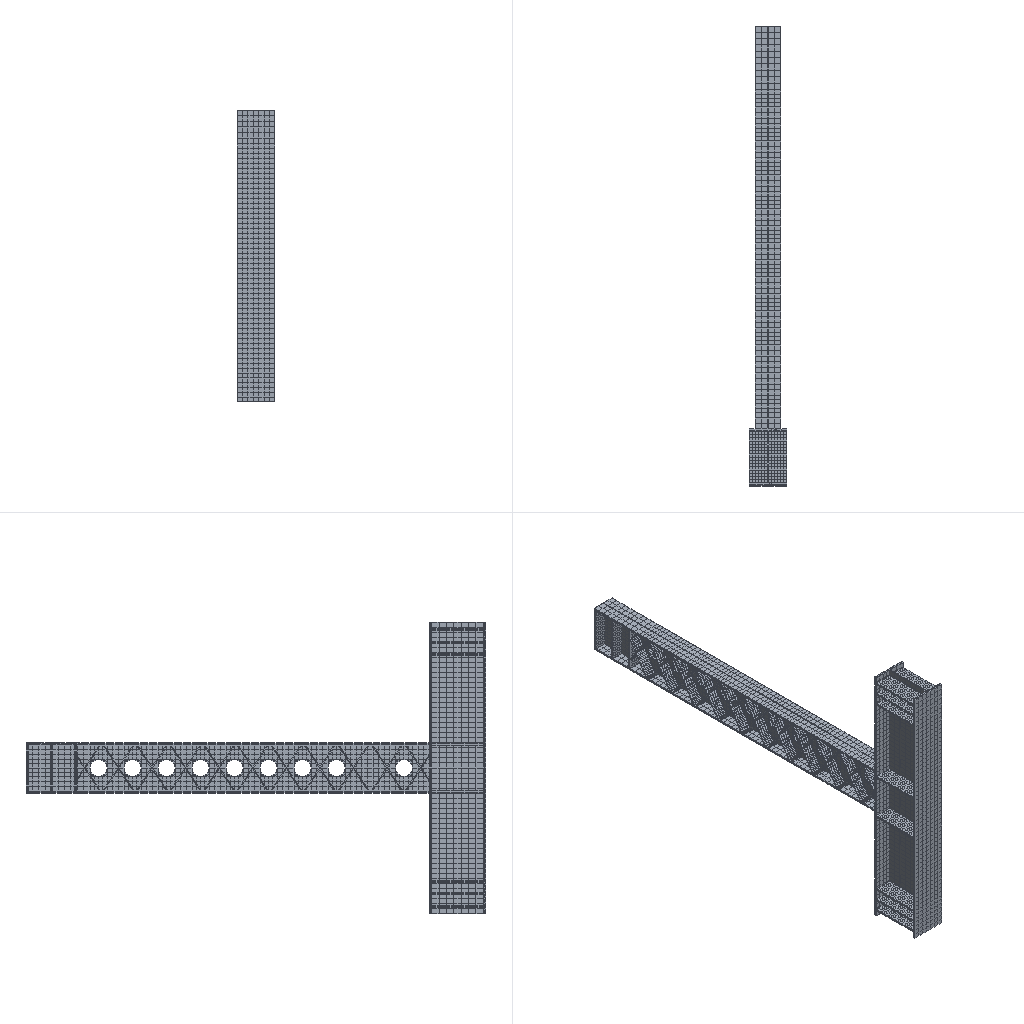Simulation study | abaqus
Set-up summary:
category,name,step,type,value,unit,region
solver,abaqus,,Abaqus/CAE 2024
units,mm-N-s-tonne (MPa),,inferred,E=200000 density=7.85e-09
analysis,Step-1,,buckling,n_modes=5
mesh,nodes,,,29001
mesh,elements,,,16108
element_type,C3D8R,,,16108
material,q235b,,E,200000
material,q235b,,nu,0.2
material,q235b,,density,7.85e-09
material,q235b,,yield,400
material,q235b,,behaviors,plastic
section,q235b,,solid section,,,Set-6
section,q235b,,solid section,,,Set-7
section,q235b,,solid section,,,Set-1
section,q235b,,solid section,,,Set-2
section,q235b,,solid section,,,Set-3
section,q235b,,solid section,,,Set-5
section,q235b,,solid section,,,Set-4
bc,BC-1,initial,fixed,"[dofs=ry,rz,x,y,z n=5]",,Set-4
bc,BC-2,initial,fixed,"[dofs=ry,rz,x,y n=4]",,Set-5
bc,BC-3,initial,fixed,[dofs=x],,Set-9
bc,BC-4,initial,fixed,[dofs=x],,Set-7
bc,BC-1,Step-1,fixed,"[dofs=ry,rz,x,y,z n=5]",,Set-4
bc,,Step-1,fixed,"[dofs=ry,rz,x,y,z n=5]",,Set-4
bc,BC-2,Step-1,fixed,"[dofs=ry,rz,x,y n=4]",,Set-5
bc,,Step-1,fixed,"[dofs=ry,rz,x,y n=4]",,Set-5
bc,BC-3,Step-1,fixed,[dofs=x],,Set-9
bc,,Step-1,fixed,[dofs=x],,Set-9
bc,BC-4,Step-1,fixed,[dofs=x],,Set-7
bc,,Step-1,fixed,[dofs=x],,Set-7
bc,BC-5,Step-1,displacement,-13 [dofs=z],,Set-8
bc,,Step-1,displacement,-13 [dofs=z],,Set-8
contact,Constraint-1,initial,tie,,,_PickedSurf141 / s_Surf-1
contact,Constraint-2,initial,tie,,,_PickedSurf142 / s_Surf-3
contact,Constraint-3,initial,tie,,,_PickedSurf143 / s_Surf-5
contact,Constraint-4,initial,tie,,,s_Surf-7 / m_Surf-7
contact,Constraint-5,initial,tie,,,s_Surf-9 / m_Surf-9
contact,Constraint-10,initial,tie,,,Surf-15 / s_Surf-5
contact,Constraint-11,initial,tie,,,s_Surf-20 / Surf-16
contact,Constraint-12,initial,tie,,,Surf-18 / s_Surf-24
contact,Constraint-13,initial,tie,,,s_Surf-5 / Surf-19
contact,Constraint-14,initial,tie,,,s_Surf-25 / Surf-20
contact,Constraint-15,initial,tie,,,Surf-23 / s_Surf-17
constraint,coupling,,,3
Abaqus input file, long lists of numbers shortened:
*Heading
** Job name: deck Model name: buqiangban-13-motai
** Generated by: Abaqus/CAE 2024
*Preprint, echo=NO, model=NO, history=NO, contact=NO
**
** PARTS
**
*Part, name=Part-1
*Node
      1,         154.,         511.,        1158.
      2,         250.,         511.,        1158.
** (463 more lines like these left out)
*Element, type=C3D8R
 1,  54, 201, 385, 193,   1,  25, 169,  38
 2, 201, 202, 386, 385,  25,  26, 170, 169
** (238 more lines like these left out)
*Nset, nset=Set-6, generate
   1,  465,    1
*Elset, elset=Set-6, generate
   1,  240,    1
** Section: q235b
*Solid Section, elset=Set-6, material=q235b
,
*End Part
**
*Part, name=Part-22
*Node
      1,         154.,   779.425,        1158.
      2,         250.,   779.425,        1158.
** (553 more lines like these left out)
*Element, type=C3D8R
 1,  66, 249, 457, 235,   1,  25, 193,  44
 2, 249, 250, 458, 457,  25,  26, 194, 193
** (286 more lines like these left out)
*Nset, nset=Set-7, generate
   1,  555,    1
*Elset, elset=Set-7, generate
   1,  288,    1
** Section: q235b
*Solid Section, elset=Set-7, material=q235b
,
*End Part
**
*Part, name=h400
*Node
      1,           0.,          16.,        507.5
      2,          96.,          16.,        507.5
** (5923 more lines like these left out)
*Element, type=C3D8R
 1,  631, 2752, 5141, 2734,    1,  590, 2716,  609
 2, 2752,  633, 2743, 5141,  590,    2,  591, 2716
** (3618 more lines like these left out)
*Nset, nset=Set-1, generate
    1,  5925,     1
*Elset, elset=Set-1, generate
    1,  3620,     1
** Section: q235b
*Solid Section, elset=Set-1, material=q235b
,
*End Part
**
*Part, name=h450
*Node
      1,         155.,         430.,        2316.
      2,         155.,          20.,        2316.
** (4069 more lines like these left out)
*Element, type=C3D8R
  1,  282, 1595, 2989, 1481,    1,   29,  797,  154
  2, 1595, 1596, 2990, 2989,   29,   30,  798,  797
** (2550 more lines like these left out)
*Nset, nset=Set-2, generate
    1,  4071,     1
*Elset, elset=Set-2, generate
    1,  2552,     1
** Section: q235b
*Solid Section, elset=Set-2, material=q235b
,
*End Part
**
*Part, name=jiajinlei20
*Node
      1,          96.,         368.,          20.
      2,          96.,   343.467,          20.
** (238 more lines like these left out)
*Element, type=C3D8R
  1,  49,  50,  66,  65,   1,   2,  18,  17
  2,  50,  51,  67,  66,   2,   3,  19,  18
** (118 more lines like these left out)
*Nset, nset=Set-3, generate
   1,  240,    1
*Elset, elset=Set-3, generate
   1,  120,    1
** Section: q235b
*Solid Section, elset=Set-3, material=q235b
,
*End Part
**
*Part, name=jiajinlei20di
*Node
      1,        112.5,         225.,          20.
      2,        112.5,      199.375,          20.
** (355 more lines like these left out)
*Element, type=C3D8R
  1,  52,  53,  70,  69,   1,   2,  19,  18
  2,  53,  54,  71,  70,   2,   3,  20,  19
** (190 more lines like these left out)
*Nset, nset=Set-5, generate
   1,  357,    1
*Elset, elset=Set-5, generate
   1,  192,    1
** Section: q235b
*Solid Section, elset=Set-5, material=q235b
,
*End Part
**
*Part, name=jiajinlie16
*Node
      1,        187.5,         375.,          16.
      2,        187.5,      349.375,          16.
** (355 more lines like these left out)
*Element, type=C3D8R
  1,  52,  53,  70,  69,   1,   2,  19,  18
  2,  53,  54,  71,  70,   2,   3,  20,  19
** (190 more lines like these left out)
*Nset, nset=Set-4, generate
   1,  357,    1
*Elset, elset=Set-4, generate
   1,  192,    1
** Section: q235b
*Solid Section, elset=Set-4, material=q235b
,
*End Part
**
**
** ASSEMBLY
**
*Assembly, name=Assembly
**
*Instance, name=h450, part=h450
*End Instance
**
*Instance, name=jiajinlie16-1, part=jiajinlie16
       112.5,          55.,        2250.
*End Instance
**
*Instance, name=jiajinlie16-1-lin-1-2, part=jiajinlie16
       112.5,          55.,        2150.
*End Instance
**
*Instance, name=jiajinlie16-1-lin-1-3, part=jiajinlie16
       112.5,          55.,        2050.
*End Instance
**
*Instance, name=jiajinlie16-1-lin-1-6, part=jiajinlie16
       112.5,          55.,          50.
*End Instance
**
*Instance, name=jiajinlie16-1-lin-1-7, part=jiajinlie16
       112.5,          55.,         150.
*End Instance
**
*Instance, name=jiajinlie16-1-lin-1-8, part=jiajinlie16
       112.5,          55.,         250.
*End Instance
**
*Instance, name=jiajinlie16-1-lin-1-2-1, part=jiajinlie16
       -42.5,          55.,        2250.
*End Instance
**
*Instance, name=jiajinlie16-1-lin-1-2-lin-1-2, part=jiajinlie16
       -42.5,          55.,        2150.
*End Instance
**
*Instance, name=jiajinlie16-1-lin-1-8-lin-1-2, part=jiajinlie16
       -42.5,          55.,         250.
*End Instance
**
*Instance, name=jiajinlie16-1-lin-1-6-lin-1-2, part=jiajinlie16
       -42.5,          55.,          50.
*End Instance
**
*Instance, name=jiajinlie16-1-lin-1-3-lin-1-2, part=jiajinlie16
       -42.5,          55.,        2050.
*End Instance
**
*Instance, name=jiajinlie16-1-lin-1-7-lin-1-2, part=jiajinlie16
       -42.5,          55.,         150.
*End Instance
**
*Instance, name=h400, part=h400
         50.,        3650.,         958.
         50.,        3650.,         958., 51.,        3650.,         958., 90.
*End Instance
**
*Instance, name=jiajinlei20-1, part=jiajinlei20
        154.,        3650.,         974.
        154.,        3650.,         974., 155.,        3650.,         974., 90.
*End Instance
**
*Instance, name=jiajinlei20-1-lin-1-2, part=jiajinlei20
        154.,        3460.,         974.
        154.,        3460.,         974., 155.,        3460.,         974., 90.
*End Instance
**
*Instance, name=jiajinlei20-1-lin-1-3, part=jiajinlei20
        154.,        3270.,         974.
        154.,        3270.,         974., 155.,        3270.,         974., 90.
*End Instance
**
*Instance, name=jiajinlei20-1-lin-1-2-1, part=jiajinlei20
         50.,        3650.,         974.
         50.,        3650.,         974., 51.,        3650.,         974., 90.
*End Instance
**
*Instance, name=jiajinlei20-1-lin-1-2-lin-1-2, part=jiajinlei20
         50.,        3460.,         974.
         50.,        3460.,         974., 51.,        3460.,         974., 90.
*End Instance
**
*Instance, name=jiajinlei20-1-lin-1-3-lin-1-2, part=jiajinlei20
         50.,        3270.,         974.
         50.,        3270.,         974., 51.,        3270.,         974., 90.
*End Instance
**
*Instance, name=Part-1-1, part=Part-1
*End Instance
**
*Instance, name=Part-22-1, part=Part-22
*End Instance
**
*Instance, name=Part-22-1-lin-2-1, part=Part-22
          0.,     266.575,           0.
*End Instance
**
*Instance, name=Part-22-1-lin-2-1-lin-2-1, part=Part-22
          0.,     533.15,           0.
*End Instance
**
*Instance, name=Part-22-1-lin-2-1-lin-3-1, part=Part-22
          0.,     799.724,           0.
*End Instance
**
*Instance, name=Part-22-1-lin-2-1-lin-4-1, part=Part-22
          0.,    1066.299,           0.
*End Instance
**
*Instance, name=Part-22-1-lin-2-1-lin-5-1, part=Part-22
          0.,     1332.874,           0.
*End Instance
**
*Instance, name=Part-22-1-lin-2-1-lin-6-1, part=Part-22
          0.,    1599.449,           0.
*End Instance
**
*Instance, name=Part-22-1-lin-2-1-lin-7-1, part=Part-22
          0.,    1866.024,           0.
*End Instance
**
*Instance, name=Part-22-1-lin-2-1-lin-8-1, part=Part-22
          0.,    2132.598,           0.
*End Instance
**
*Instance, name=Part-1-2, part=Part-1
        404.,        3700.,           0.
        404.,        3700.,           0.,         404.,        3700.,           1.,         180.
*End Instance
**
*Instance, name=Part-1-2-lin-1-2, part=Part-1
        300.,        3700.,           0.
        300.,        3700.,           0.,         300.,        3700.,           1.,         180.
*End Instance
**
*Instance, name=Part-22-1-lin-2-1-lin-8-1-lin-1-2, part=Part-22
       -104.,    2132.598,           0.
*End Instance
**
*Instance, name=Part-22-1-lin-2-1-lin-7-1-lin-1-2, part=Part-22
       -104.,    1866.024,           0.
*End Instance
**
*Instance, name=Part-22-1-lin-2-1-lin-6-1-lin-1-2, part=Part-22
       -104.,    1599.449,           0.
*End Instance
**
*Instance, name=Part-22-1-lin-2-1-lin-5-1-lin-1-2, part=Part-22
       -104.,     1332.874,           0.
*End Instance
**
*Instance, name=Part-22-1-lin-2-1-lin-4-1-lin-1-2, part=Part-22
       -104.,    1066.299,           0.
*End Instance
**
*Instance, name=Part-22-1-lin-2-1-lin-2-1-lin-1-2, part=Part-22
       -104.,     533.15,           0.
*End Instance
**
*Instance, name=Part-22-1-lin-1-2, part=Part-22
       -104.,           0.,           0.
*End Instance
**
*Instance, name=Part-22-1-lin-2-1-lin-1-2, part=Part-22
       -104.,     266.575,           0.
*End Instance
**
*Instance, name=Part-22-1-lin-2-1-lin-3-1-lin-1-2, part=Part-22
       -104.,     799.724,           0.
*End Instance
**
*Instance, name=Part-1-1-lin-1-2, part=Part-1
       -104.,           0.,           0.
*End Instance
**
*Instance, name=jiajinlei20di-1, part=jiajinlei20di
       187.5,         205.,        1340.
*End Instance
**
*Instance, name=jiajinlei20di-2, part=jiajinlei20di
       187.5,         205.,         956.
*End Instance
**
*Instance, name=jiajinlei20di-1-lin-1-2, part=jiajinlei20di
        32.5,         205.,        1340.
*End Instance
**
*Instance, name=jiajinlei20di-2-lin-1-2, part=jiajinlei20di
        32.5,         205.,         956.
*End Instance
**
*Node
      1,         150.,           0.,        2183.
*Node
      2,         150.,           0.,         133.
*Node
      3,         150.,        3450.,        1358.
*Nset, nset=Set-4
 1,
*Nset, nset=Set-5
 2,
*Nset, nset=Set-6, instance=jiajinlie16-1, generate
  1,  51,   1
*Nset, nset=Set-6, instance=jiajinlie16-1-lin-1-2, generate
  1,  51,   1
*Nset, nset=Set-6, instance=jiajinlie16-1-lin-1-3, generate
  1,  51,   1
*Nset, nset=Set-6, instance=jiajinlie16-1-lin-1-7, generate
  1,  51,   1
*Nset, nset=Set-6, instance=jiajinlie16-1-lin-1-2-1, generate
 307,  357,    1
*Nset, nset=Set-6, instance=jiajinlie16-1-lin-1-6-lin-1-2, generate
 307,  357,    1
*Nset, nset=Set-6, instance=jiajinlie16-1-lin-1-6, generate
  1,  51,   1
*Nset, nset=Set-6, instance=jiajinlie16-1-lin-1-8, generate
  1,  51,   1
*Nset, nset=Set-6, instance=jiajinlie16-1-lin-1-7-lin-1-2, generate
 307,  357,    1
*Nset, nset=Set-6, instance=jiajinlie16-1-lin-1-8-lin-1-2, generate
 307,  357,    1
*Nset, nset=Set-6, instance=jiajinlie16-1-lin-1-2-lin-1-2, generate
 307,  357,    1
*Nset, nset=Set-6, instance=jiajinlie16-1-lin-1-3-lin-1-2, generate
 307,  357,    1
*Elset, elset=Set-6, instance=jiajinlie16-1, generate
  1,  32,   1
*Elset, elset=Set-6, instance=jiajinlie16-1-lin-1-2, generate
  1,  32,   1
*Elset, elset=Set-6, instance=jiajinlie16-1-lin-1-3, generate
  1,  32,   1
*Elset, elset=Set-6, instance=jiajinlie16-1-lin-1-7, generate
  1,  32,   1
*Elset, elset=Set-6, instance=jiajinlie16-1-lin-1-2-1, generate
 161,  192,    1
*Elset, elset=Set-6, instance=jiajinlie16-1-lin-1-6-lin-1-2, generate
 161,  192,    1
*Elset, elset=Set-6, instance=jiajinlie16-1-lin-1-6, generate
  1,  32,   1
*Elset, elset=Set-6, instance=jiajinlie16-1-lin-1-8, generate
  1,  32,   1
*Elset, elset=Set-6, instance=jiajinlie16-1-lin-1-7-lin-1-2, generate
 161,  192,    1
*Elset, elset=Set-6, instance=jiajinlie16-1-lin-1-8-lin-1-2, generate
 161,  192,    1
*Elset, elset=Set-6, instance=jiajinlie16-1-lin-1-2-lin-1-2, generate
 161,  192,    1
*Elset, elset=Set-6, instance=jiajinlie16-1-lin-1-3-lin-1-2, generate
 161,  192,    1
*Nset, nset=Set-7, instance=jiajinlei20-1, generate
  1,  48,   1
*Nset, nset=Set-7, instance=jiajinlei20-1-lin-1-2, generate
  1,  48,   1
*Nset, nset=Set-7, instance=jiajinlei20-1-lin-1-2-1, generate
 193,  240,    1
*Nset, nset=Set-7, instance=jiajinlei20-1-lin-1-3-lin-1-2, generate
 193,  240,    1
*Nset, nset=Set-7, instance=jiajinlei20-1-lin-1-3, generate
  1,  48,   1
*Nset, nset=Set-7, instance=jiajinlei20-1-lin-1-2-lin-1-2, generate
 193,  240,    1
*Elset, elset=Set-7, instance=jiajinlei20-1, generate
  1,  30,   1
*Elset, elset=Set-7, instance=jiajinlei20-1-lin-1-2, generate
  1,  30,   1
*Elset, elset=Set-7, instance=jiajinlei20-1-lin-1-2-1, generate
  91,  120,    1
*Elset, elset=Set-7, instance=jiajinlei20-1-lin-1-3-lin-1-2, generate
  91,  120,    1
*Elset, elset=Set-7, instance=jiajinlei20-1-lin-1-3, generate
  1,  30,   1
*Elset, elset=Set-7, instance=jiajinlei20-1-lin-1-2-lin-1-2, generate
  91,  120,    1
*Nset, nset=Set-8
 3,
*Nset, nset=Set-9, instance=jiajinlie16-1, generate
  1,  51,   1
*Nset, nset=Set-9, instance=jiajinlie16-1-lin-1-2, generate
  1,  51,   1
*Nset, nset=Set-9, instance=jiajinlie16-1-lin-1-3, generate
  1,  51,   1
*Nset, nset=Set-9, instance=jiajinlie16-1-lin-1-7, generate
  1,  51,   1
*Nset, nset=Set-9, instance=jiajinlie16-1-lin-1-2-1, generate
 307,  357,    1
*Nset, nset=Set-9, instance=jiajinlie16-1-lin-1-6-lin-1-2, generate
 307,  357,    1
*Nset, nset=Set-9, instance=jiajinlie16-1-lin-1-6, generate
  1,  51,   1
*Nset, nset=Set-9, instance=jiajinlie16-1-lin-1-8, generate
  1,  51,   1
*Nset, nset=Set-9, instance=jiajinlie16-1-lin-1-7-lin-1-2, generate
 307,  357,    1
*Nset, nset=Set-9, instance=jiajinlie16-1-lin-1-8-lin-1-2, generate
 307,  357,    1
*Nset, nset=Set-9, instance=jiajinlie16-1-lin-1-2-lin-1-2, generate
 307,  357,    1
*Nset, nset=Set-9, instance=jiajinlie16-1-lin-1-3-lin-1-2, generate
 307,  357,    1
*Nset, nset=Set-9, instance=jiajinlei20di-1, generate
  1,  51,   1
*Nset, nset=Set-9, instance=jiajinlei20di-1-lin-1-2, generate
 307,  357,    1
*Nset, nset=Set-9, instance=jiajinlei20di-2, generate
  1,  51,   1
*Nset, nset=Set-9, instance=jiajinlei20di-2-lin-1-2, generate
 307,  357,    1
*Elset, elset=Set-9, instance=jiajinlie16-1, generate
  1,  32,   1
*Elset, elset=Set-9, instance=jiajinlie16-1-lin-1-2, generate
  1,  32,   1
*Elset, elset=Set-9, instance=jiajinlie16-1-lin-1-3, generate
  1,  32,   1
*Elset, elset=Set-9, instance=jiajinlie16-1-lin-1-7, generate
  1,  32,   1
*Elset, elset=Set-9, instance=jiajinlie16-1-lin-1-2-1, generate
 161,  192,    1
*Elset, elset=Set-9, instance=jiajinlie16-1-lin-1-6-lin-1-2, generate
 161,  192,    1
*Elset, elset=Set-9, instance=jiajinlie16-1-lin-1-6, generate
  1,  32,   1
*Elset, elset=Set-9, instance=jiajinlie16-1-lin-1-8, generate
  1,  32,   1
*Elset, elset=Set-9, instance=jiajinlie16-1-lin-1-7-lin-1-2, generate
 161,  192,    1
*Elset, elset=Set-9, instance=jiajinlie16-1-lin-1-8-lin-1-2, generate
 161,  192,    1
*Elset, elset=Set-9, instance=jiajinlie16-1-lin-1-2-lin-1-2, generate
 161,  192,    1
*Elset, elset=Set-9, instance=jiajinlie16-1-lin-1-3-lin-1-2, generate
 161,  192,    1
*Elset, elset=Set-9, instance=jiajinlei20di-1, generate
  1,  32,   1
*Elset, elset=Set-9, instance=jiajinlei20di-1-lin-1-2, generate
 161,  192,    1
*Elset, elset=Set-9, instance=jiajinlei20di-2, generate
  1,  32,   1
*Elset, elset=Set-9, instance=jiajinlei20di-2-lin-1-2, generate
 161,  192,    1
*Nset, nset=m_Set-1
 3,
*Nset, nset=m_Set-2
 1,
*Nset, nset=m_Set-3
 2,
*Elset, elset=_Surf-15_S5, internal, instance=Part-1-1
  17,  18,  19,  20,  37,  38,  39,  40, 173, 174, 175, 176, 237, 238, 239, 240
*Surface, type=ELEMENT, name=Surf-15
_Surf-15_S5, S5
*Elset, elset=_Surf-16_S5, internal, instance=Part-1-2
  17,  18,  19,  20,  37,  38,  39,  40, 173, 174, 175, 176, 237, 238, 239, 240
*Surface, type=ELEMENT, name=Surf-16
_Surf-16_S5, S5
*Elset, elset=_Surf-18_S4, internal, instance=Part-1-2-lin-1-2, generate
  44,  240,    4
*Elset, elset=_Surf-18_S4, internal, instance=Part-22-1-lin-2-1-lin-8-1-lin-1-2, generate
   4,  216,    4
*Elset, elset=_Surf-18_S4, internal, instance=Part-22-1-lin-2-1-lin-6-1-lin-1-2, generate
   4,  216,    4
*Elset, elset=_Surf-18_S4, internal, instance=Part-22-1-lin-2-1-lin-4-1-lin-1-2, generate
   4,  216,    4
*Elset, elset=_Surf-18_S4, internal, instance=Part-22-1-lin-2-1-lin-3-1-lin-1-2, generate
   4,  216,    4
*Elset, elset=_Surf-18_S4, internal, instance=Part-22-1-lin-1-2, generate
   4,  216,    4
*Elset, elset=_Surf-18_S4, internal, instance=Part-22-1-lin-2-1-lin-7-1-lin-1-2, generate
   4,  216,    4
*Elset, elset=_Surf-18_S4, internal, instance=Part-22-1-lin-2-1-lin-2-1-lin-1-2, generate
   4,  216,    4
*Elset, elset=_Surf-18_S4, internal, instance=Part-1-1-lin-1-2, generate
  4,  40,   4
*Elset, elset=_Surf-18_S4, internal, instance=Part-22-1-lin-2-1-lin-5-1-lin-1-2, generate
   4,  216,    4
*Elset, elset=_Surf-18_S4, internal, instance=Part-22-1-lin-2-1-lin-1-2, generate
   4,  216,    4
*Elset, elset=_Surf-18_S3, internal, instance=Part-1-2-lin-1-2
 113, 114, 115, 116, 177, 178, 179, 180
*Elset, elset=_Surf-18_S3, internal, instance=Part-22-1-lin-2-1-lin-8-1-lin-1-2
  65,  66,  67,  68, 141, 142, 143, 144
*Elset, elset=_Surf-18_S3, internal, instance=Part-22-1-lin-2-1-lin-6-1-lin-1-2
  65,  66,  67,  68, 141, 142, 143, 144
*Elset, elset=_Surf-18_S3, internal, instance=Part-22-1-lin-2-1-lin-4-1-lin-1-2
  65,  66,  67,  68, 141, 142, 143, 144
*Elset, elset=_Surf-18_S3, internal, instance=Part-22-1-lin-2-1-lin-3-1-lin-1-2
  65,  66,  67,  68, 141, 142, 143, 144
*Elset, elset=_Surf-18_S3, internal, instance=Part-22-1-lin-1-2
  65,  66,  67,  68, 141, 142, 143, 144
*Elset, elset=_Surf-18_S3, internal, instance=Part-22-1-lin-2-1-lin-7-1-lin-1-2
  65,  66,  67,  68, 141, 142, 143, 144
*Elset, elset=_Surf-18_S3, internal, instance=Part-22-1-lin-2-1-lin-2-1-lin-1-2
  65,  66,  67,  68, 141, 142, 143, 144
*Elset, elset=_Surf-18_S3, internal, instance=Part-1-1-lin-1-2
 113, 114, 115, 116, 177, 178, 179, 180
*Elset, elset=_Surf-18_S3, internal, instance=Part-22-1-lin-2-1-lin-5-1-lin-1-2
  65,  66,  67,  68, 141, 142, 143, 144
*Elset, elset=_Surf-18_S3, internal, instance=Part-22-1-lin-2-1-lin-1-2
  65,  66,  67,  68, 141, 142, 143, 144
*Elset, elset=_Surf-18_S5, internal, instance=Part-1-2-lin-1-2
  73,  74,  75,  76, 109, 110, 111, 112
*Elset, elset=_Surf-18_S5, internal, instance=Part-22-1-lin-2-1-lin-8-1-lin-1-2
  29,  30,  31,  32,  61,  62,  63,  64, 137, 138, 139, 140, 213, 214, 215, 216
 249, 250, 251, 252, 285, 286, 287, 288
*Elset, elset=_Surf-18_S5, internal, instance=Part-22-1-lin-2-1-lin-6-1-lin-1-2
  29,  30,  31,  32,  61,  62,  63,  64, 137, 138, 139, 140, 213, 214, 215, 216
 249, 250, 251, 252, 285, 286, 287, 288
*Elset, elset=_Surf-18_S5, internal, instance=Part-22-1-lin-2-1-lin-4-1-lin-1-2
  29,  30,  31,  32,  61,  62,  63,  64, 137, 138, 139, 140, 213, 214, 215, 216
 249, 250, 251, 252, 285, 286, 287, 288
*Elset, elset=_Surf-18_S5, internal, instance=Part-22-1-lin-2-1-lin-3-1-lin-1-2
  29,  30,  31,  32,  61,  62,  63,  64, 137, 138, 139, 140, 213, 214, 215, 216
 249, 250, 251, 252, 285, 286, 287, 288
*Elset, elset=_Surf-18_S5, internal, instance=Part-22-1-lin-1-2
  29,  30,  31,  32,  61,  62,  63,  64, 137, 138, 139, 140, 213, 214, 215, 216
 249, 250, 251, 252, 285, 286, 287, 288
*Elset, elset=_Surf-18_S5, internal, instance=Part-22-1-lin-2-1-lin-7-1-lin-1-2
  29,  30,  31,  32,  61,  62,  63,  64, 137, 138, 139, 140, 213, 214, 215, 216
 249, 250, 251, 252, 285, 286, 287, 288
*Elset, elset=_Surf-18_S5, internal, instance=Part-22-1-lin-2-1-lin-2-1-lin-1-2
  29,  30,  31,  32,  61,  62,  63,  64, 137, 138, 139, 140, 213, 214, 215, 216
 249, 250, 251, 252, 285, 286, 287, 288
*Elset, elset=_Surf-18_S5, internal, instance=Part-1-1-lin-1-2
  73,  74,  75,  76, 109, 110, 111, 112
*Elset, elset=_Surf-18_S5, internal, instance=Part-22-1-lin-2-1-lin-5-1-lin-1-2
  29,  30,  31,  32,  61,  62,  63,  64, 137, 138, 139, 140, 213, 214, 215, 216
 249, 250, 251, 252, 285, 286, 287, 288
*Elset, elset=_Surf-18_S5, internal, instance=Part-22-1-lin-2-1-lin-1-2
  29,  30,  31,  32,  61,  62,  63,  64, 137, 138, 139, 140, 213, 214, 215, 216
 249, 250, 251, 252, 285, 286, 287, 288
*Elset, elset=_Surf-18_S6, internal, instance=Part-1-2-lin-1-2, generate
  1,  37,   4
*Elset, elset=_Surf-18_S6, internal, instance=Part-22-1-lin-2-1-lin-8-1-lin-1-2, generate
 217,  285,    4
*Elset, elset=_Surf-18_S6, internal, instance=Part-22-1-lin-2-1-lin-6-1-lin-1-2, generate
 217,  285,    4
*Elset, elset=_Surf-18_S6, internal, instance=Part-22-1-lin-2-1-lin-4-1-lin-1-2, generate
 217,  285,    4
*Elset, elset=_Surf-18_S6, internal, instance=Part-22-1-lin-2-1-lin-3-1-lin-1-2, generate
 217,  285,    4
*Elset, elset=_Surf-18_S6, internal, instance=Part-22-1-lin-1-2, generate
 217,  285,    4
*Elset, elset=_Surf-18_S6, internal, instance=Part-22-1-lin-2-1-lin-7-1-lin-1-2, generate
 217,  285,    4
*Elset, elset=_Surf-18_S6, internal, instance=Part-22-1-lin-2-1-lin-2-1-lin-1-2, generate
 217,  285,    4
*Elset, elset=_Surf-18_S6, internal, instance=Part-1-1-lin-1-2, generate
  41,  237,    4
*Elset, elset=_Surf-18_S6, internal, instance=Part-22-1-lin-2-1-lin-5-1-lin-1-2, generate
 217,  285,    4
*Elset, elset=_Surf-18_S6, internal, instance=Part-22-1-lin-2-1-lin-1-2, generate
 217,  285,    4
*Surface, type=ELEMENT, name=Surf-18
_Surf-18_S4, S4
_Surf-18_S3, S3
_Surf-18_S6, S6
_Surf-18_S5, S5
*Elset, elset=_Surf-19_S5, internal, instance=Part-1-1-lin-1-2
  17,  18,  19,  20,  37,  38,  39,  40, 173, 174, 175, 176, 237, 238, 239, 240
*Surface, type=ELEMENT, name=Surf-19
_Surf-19_S5, S5
*Elset, elset=_Surf-20_S5, internal, instance=Part-1-2-lin-1-2
  17,  18,  19,  20,  37,  38,  39,  40, 173, 174, 175, 176, 237, 238, 239, 240
*Surface, type=ELEMENT, name=Surf-20
_Surf-20_S5, S5
*Elset, elset=_Surf-23_S4, internal, instance=Part-1-1, generate
  44,  240,    4
*Elset, elset=_Surf-23_S4, internal, instance=Part-22-1, generate
 220,  288,    4
*Elset, elset=_Surf-23_S4, internal, instance=Part-22-1-lin-2-1, generate
 220,  288,    4
*Elset, elset=_Surf-23_S4, internal, instance=Part-22-1-lin-2-1-lin-3-1, generate
 220,  288,    4
*Elset, elset=_Surf-23_S4, internal, instance=Part-22-1-lin-2-1-lin-7-1, generate
 220,  288,    4
*Elset, elset=_Surf-23_S4, internal, instance=Part-22-1-lin-2-1-lin-5-1, generate
 220,  288,    4
*Elset, elset=_Surf-23_S4, internal, instance=Part-1-2, generate
  4,  40,   4
*Elset, elset=_Surf-23_S4, internal, instance=Part-22-1-lin-2-1-lin-2-1, generate
 220,  288,    4
*Elset, elset=_Surf-23_S4, internal, instance=Part-22-1-lin-2-1-lin-4-1, generate
 220,  288,    4
*Elset, elset=_Surf-23_S4, internal, instance=Part-22-1-lin-2-1-lin-8-1, generate
 220,  288,    4
*Elset, elset=_Surf-23_S4, internal, instance=Part-22-1-lin-2-1-lin-6-1, generate
 220,  288,    4
*Elset, elset=_Surf-23_S3, internal, instance=Part-1-1
 113, 114, 115, 116, 177, 178, 179, 180
*Elset, elset=_Surf-23_S3, internal, instance=Part-22-1
  65,  66,  67,  68, 141, 142, 143, 144
*Elset, elset=_Surf-23_S3, internal, instance=Part-22-1-lin-2-1
  65,  66,  67,  68, 141, 142, 143, 144
*Elset, elset=_Surf-23_S3, internal, instance=Part-22-1-lin-2-1-lin-3-1
  65,  66,  67,  68, 141, 142, 143, 144
*Elset, elset=_Surf-23_S3, internal, instance=Part-22-1-lin-2-1-lin-7-1
  65,  66,  67,  68, 141, 142, 143, 144
*Elset, elset=_Surf-23_S3, internal, instance=Part-22-1-lin-2-1-lin-5-1
  65,  66,  67,  68, 141, 142, 143, 144
*Elset, elset=_Surf-23_S3, internal, instance=Part-1-2
 113, 114, 115, 116, 177, 178, 179, 180
*Elset, elset=_Surf-23_S3, internal, instance=Part-22-1-lin-2-1-lin-2-1
  65,  66,  67,  68, 141, 142, 143, 144
*Elset, elset=_Surf-23_S3, internal, instance=Part-22-1-lin-2-1-lin-4-1
  65,  66,  67,  68, 141, 142, 143, 144
*Elset, elset=_Surf-23_S3, internal, instance=Part-22-1-lin-2-1-lin-8-1
  65,  66,  67,  68, 141, 142, 143, 144
*Elset, elset=_Surf-23_S3, internal, instance=Part-22-1-lin-2-1-lin-6-1
  65,  66,  67,  68, 141, 142, 143, 144
*Elset, elset=_Surf-23_S5, internal, instance=Part-1-1
  73,  74,  75,  76, 109, 110, 111, 112
*Elset, elset=_Surf-23_S5, internal, instance=Part-22-1
  29,  30,  31,  32,  61,  62,  63,  64, 137, 138, 139, 140, 213, 214, 215, 216
 249, 250, 251, 252, 285, 286, 287, 288
*Elset, elset=_Surf-23_S5, internal, instance=Part-22-1-lin-2-1
  29,  30,  31,  32,  61,  62,  63,  64, 137, 138, 139, 140, 213, 214, 215, 216
 249, 250, 251, 252, 285, 286, 287, 288
*Elset, elset=_Surf-23_S5, internal, instance=Part-22-1-lin-2-1-lin-3-1
  29,  30,  31,  32,  61,  62,  63,  64, 137, 138, 139, 140, 213, 214, 215, 216
 249, 250, 251, 252, 285, 286, 287, 288
*Elset, elset=_Surf-23_S5, internal, instance=Part-22-1-lin-2-1-lin-7-1
  29,  30,  31,  32,  61,  62,  63,  64, 137, 138, 139, 140, 213, 214, 215, 216
 249, 250, 251, 252, 285, 286, 287, 288
*Elset, elset=_Surf-23_S5, internal, instance=Part-22-1-lin-2-1-lin-5-1
  29,  30,  31,  32,  61,  62,  63,  64, 137, 138, 139, 140, 213, 214, 215, 216
 249, 250, 251, 252, 285, 286, 287, 288
*Elset, elset=_Surf-23_S5, internal, instance=Part-1-2
  73,  74,  75,  76, 109, 110, 111, 112
*Elset, elset=_Surf-23_S5, internal, instance=Part-22-1-lin-2-1-lin-2-1
  29,  30,  31,  32,  61,  62,  63,  64, 137, 138, 139, 140, 213, 214, 215, 216
 249, 250, 251, 252, 285, 286, 287, 288
*Elset, elset=_Surf-23_S5, internal, instance=Part-22-1-lin-2-1-lin-4-1
  29,  30,  31,  32,  61,  62,  63,  64, 137, 138, 139, 140, 213, 214, 215, 216
 249, 250, 251, 252, 285, 286, 287, 288
*Elset, elset=_Surf-23_S5, internal, instance=Part-22-1-lin-2-1-lin-8-1
  29,  30,  31,  32,  61,  62,  63,  64, 137, 138, 139, 140, 213, 214, 215, 216
 249, 250, 251, 252, 285, 286, 287, 288
*Elset, elset=_Surf-23_S5, internal, instance=Part-22-1-lin-2-1-lin-6-1
  29,  30,  31,  32,  61,  62,  63,  64, 137, 138, 139, 140, 213, 214, 215, 216
 249, 250, 251, 252, 285, 286, 287, 288
*Elset, elset=_Surf-23_S6, internal, instance=Part-1-1, generate
  1,  37,   4
*Elset, elset=_Surf-23_S6, internal, instance=Part-22-1, generate
   1,  213,    4
*Elset, elset=_Surf-23_S6, internal, instance=Part-22-1-lin-2-1, generate
   1,  213,    4
*Elset, elset=_Surf-23_S6, internal, instance=Part-22-1-lin-2-1-lin-3-1, generate
   1,  213,    4
*Elset, elset=_Surf-23_S6, internal, instance=Part-22-1-lin-2-1-lin-7-1, generate
   1,  213,    4
*Elset, elset=_Surf-23_S6, internal, instance=Part-22-1-lin-2-1-lin-5-1, generate
   1,  213,    4
*Elset, elset=_Surf-23_S6, internal, instance=Part-1-2, generate
  41,  237,    4
*Elset, elset=_Surf-23_S6, internal, instance=Part-22-1-lin-2-1-lin-2-1, generate
   1,  213,    4
*Elset, elset=_Surf-23_S6, internal, instance=Part-22-1-lin-2-1-lin-4-1, generate
   1,  213,    4
*Elset, elset=_Surf-23_S6, internal, instance=Part-22-1-lin-2-1-lin-8-1, generate
   1,  213,    4
*Elset, elset=_Surf-23_S6, internal, instance=Part-22-1-lin-2-1-lin-6-1, generate
   1,  213,    4
*Surface, type=ELEMENT, name=Surf-23
_Surf-23_S4, S4
_Surf-23_S3, S3
_Surf-23_S6, S6
_Surf-23_S5, S5
*Elset, elset=_m_Surf-1_S1, internal, instance=jiajinlie16-1, generate
 161,  192,    1
*Elset, elset=_m_Surf-1_S1, internal, instance=jiajinlie16-1-lin-1-2, generate
 161,  192,    1
*Elset, elset=_m_Surf-1_S1, internal, instance=jiajinlie16-1-lin-1-3, generate
 161,  192,    1
*Elset, elset=_m_Surf-1_S1, internal, instance=jiajinlie16-1-lin-1-7, generate
 161,  192,    1
*Elset, elset=_m_Surf-1_S1, internal, instance=jiajinlie16-1-lin-1-6, generate
 161,  192,    1
*Elset, elset=_m_Surf-1_S1, internal, instance=jiajinlie16-1-lin-1-8, generate
 161,  192,    1
*Elset, elset=_m_Surf-1_S6, internal, instance=jiajinlie16-1, generate
   1,  177,   16
*Elset, elset=_m_Surf-1_S6, internal, instance=jiajinlie16-1-lin-1-2, generate
   1,  177,   16
*Elset, elset=_m_Surf-1_S6, internal, instance=jiajinlie16-1-lin-1-3, generate
   1,  177,   16
*Elset, elset=_m_Surf-1_S6, internal, instance=jiajinlie16-1-lin-1-7, generate
   1,  177,   16
*Elset, elset=_m_Surf-1_S6, internal, instance=jiajinlie16-1-lin-1-6, generate
   1,  177,   16
*Elset, elset=_m_Surf-1_S6, internal, instance=jiajinlie16-1-lin-1-8, generate
   1,  177,   16
*Elset, elset=_m_Surf-1_S4, internal, instance=jiajinlie16-1, generate
  16,  192,   16
*Elset, elset=_m_Surf-1_S4, internal, instance=jiajinlie16-1-lin-1-2, generate
  16,  192,   16
*Elset, elset=_m_Surf-1_S4, internal, instance=jiajinlie16-1-lin-1-3, generate
  16,  192,   16
*Elset, elset=_m_Surf-1_S4, internal, instance=jiajinlie16-1-lin-1-7, generate
  16,  192,   16
*Elset, elset=_m_Surf-1_S4, internal, instance=jiajinlie16-1-lin-1-6, generate
  16,  192,   16
*Elset, elset=_m_Surf-1_S4, internal, instance=jiajinlie16-1-lin-1-8, generate
  16,  192,   16
*Surface, type=ELEMENT, name=m_Surf-1
_m_Surf-1_S1, S1
_m_Surf-1_S6, S6
_m_Surf-1_S4, S4
*Elset, elset=_m_Surf-3_S6, internal, instance=jiajinlie16-1-lin-1-2-1, generate
   1,  177,   16
*Elset, elset=_m_Surf-3_S6, internal, instance=jiajinlie16-1-lin-1-2-lin-1-2, generate
   1,  177,   16
*Elset, elset=_m_Surf-3_S6, internal, instance=jiajinlie16-1-lin-1-6-lin-1-2, generate
   1,  177,   16
*Elset, elset=_m_Surf-3_S6, internal, instance=jiajinlie16-1-lin-1-8-lin-1-2, generate
   1,  177,   16
*Elset, elset=_m_Surf-3_S6, internal, instance=jiajinlie16-1-lin-1-7-lin-1-2, generate
   1,  177,   16
*Elset, elset=_m_Surf-3_S6, internal, instance=jiajinlie16-1-lin-1-3-lin-1-2, generate
   1,  177,   16
*Elset, elset=_m_Surf-3_S2, internal, instance=jiajinlie16-1-lin-1-2-1, generate
  1,  32,   1
*Elset, elset=_m_Surf-3_S2, internal, instance=jiajinlie16-1-lin-1-2-lin-1-2, generate
  1,  32,   1
*Elset, elset=_m_Surf-3_S2, internal, instance=jiajinlie16-1-lin-1-6-lin-1-2, generate
  1,  32,   1
*Elset, elset=_m_Surf-3_S2, internal, instance=jiajinlie16-1-lin-1-8-lin-1-2, generate
  1,  32,   1
*Elset, elset=_m_Surf-3_S2, internal, instance=jiajinlie16-1-lin-1-7-lin-1-2, generate
  1,  32,   1
*Elset, elset=_m_Surf-3_S2, internal, instance=jiajinlie16-1-lin-1-3-lin-1-2, generate
  1,  32,   1
*Elset, elset=_m_Surf-3_S4, internal, instance=jiajinlie16-1-lin-1-2-1, generate
  16,  192,   16
*Elset, elset=_m_Surf-3_S4, internal, instance=jiajinlie16-1-lin-1-2-lin-1-2, generate
  16,  192,   16
*Elset, elset=_m_Surf-3_S4, internal, instance=jiajinlie16-1-lin-1-6-lin-1-2, generate
  16,  192,   16
*Elset, elset=_m_Surf-3_S4, internal, instance=jiajinlie16-1-lin-1-8-lin-1-2, generate
  16,  192,   16
*Elset, elset=_m_Surf-3_S4, internal, instance=jiajinlie16-1-lin-1-7-lin-1-2, generate
  16,  192,   16
*Elset, elset=_m_Surf-3_S4, internal, instance=jiajinlie16-1-lin-1-3-lin-1-2, generate
  16,  192,   16
*Surface, type=ELEMENT, name=m_Surf-3
_m_Surf-3_S6, S6
_m_Surf-3_S2, S2
_m_Surf-3_S4, S4
*Elset, elset=_m_Surf-5_S3, internal, instance=h400
 3305, 3306, 3463, 3464
*Elset, elset=_m_Surf-5_S5, internal, instance=h400
 1181, 1182, 1187, 1188, 2357, 2358, 2363, 2364, 2521, 2522, 2679, 2680, 2725, 2726, 2731, 2732
 3273, 3274, 3279, 3280
*Surface, type=ELEMENT, name=m_Surf-5
_m_Surf-5_S3, S3
_m_Surf-5_S5, S5
*Elset, elset=_m_Surf-7_S1, internal, instance=jiajinlei20-1, generate
  91,  120,    1
*Elset, elset=_m_Surf-7_S1, internal, instance=jiajinlei20-1-lin-1-2, generate
  91,  120,    1
*Elset, elset=_m_Surf-7_S1, internal, instance=jiajinlei20-1-lin-1-3, generate
  91,  120,    1
*Elset, elset=_m_Surf-7_S6, internal, instance=jiajinlei20-1, generate
   1,  106,   15
*Elset, elset=_m_Surf-7_S6, internal, instance=jiajinlei20-1-lin-1-2, generate
   1,  106,   15
*Elset, elset=_m_Surf-7_S6, internal, instance=jiajinlei20-1-lin-1-3, generate
   1,  106,   15
*Elset, elset=_m_Surf-7_S4, internal, instance=jiajinlei20-1, generate
  15,  120,   15
*Elset, elset=_m_Surf-7_S4, internal, instance=jiajinlei20-1-lin-1-2, generate
  15,  120,   15
*Elset, elset=_m_Surf-7_S4, internal, instance=jiajinlei20-1-lin-1-3, generate
  15,  120,   15
*Surface, type=ELEMENT, name=m_Surf-7
_m_Surf-7_S1, S1
_m_Surf-7_S6, S6
_m_Surf-7_S4, S4
*Elset, elset=_m_Surf-9_S6, internal, instance=jiajinlei20-1-lin-1-2-1, generate
   1,  106,   15
*Elset, elset=_m_Surf-9_S6, internal, instance=jiajinlei20-1-lin-1-2-lin-1-2, generate
   1,  106,   15
*Elset, elset=_m_Surf-9_S6, internal, instance=jiajinlei20-1-lin-1-3-lin-1-2, generate
   1,  106,   15
*Elset, elset=_m_Surf-9_S2, internal, instance=jiajinlei20-1-lin-1-2-1, generate
  1,  30,   1
*Elset, elset=_m_Surf-9_S2, internal, instance=jiajinlei20-1-lin-1-2-lin-1-2, generate
  1,  30,   1
*Elset, elset=_m_Surf-9_S2, internal, instance=jiajinlei20-1-lin-1-3-lin-1-2, generate
  1,  30,   1
*Elset, elset=_m_Surf-9_S4, internal, instance=jiajinlei20-1-lin-1-2-1, generate
  15,  120,   15
*Elset, elset=_m_Surf-9_S4, internal, instance=jiajinlei20-1-lin-1-2-lin-1-2, generate
  15,  120,   15
*Elset, elset=_m_Surf-9_S4, internal, instance=jiajinlei20-1-lin-1-3-lin-1-2, generate
  15,  120,   15
*Surface, type=ELEMENT, name=m_Surf-9
_m_Surf-9_S6, S6
_m_Surf-9_S2, S2
_m_Surf-9_S4, S4
*Elset, elset=_s_Surf-1_S2, internal, instance=h450
    1,    2,    3,    4,    5,    6,    7,    8,    9,   10,   11,   12,   13,   14,   15,   16
   17,   18,   19,   20,   21,   22,   23,   24,   25,   26,   27,   28,   29,   30,   31,   32
** (31 more lines like these left out)
*Elset, elset=_s_Surf-1_S1, internal, instance=h450
 2147, 2148, 2154, 2155, 2161, 2162, 2168, 2169, 2175, 2176, 2182, 2183, 2189, 2190, 2196, 2197
 2203, 2204, 2210, 2211, 2217, 2218, 2224, 2225, 2231, 2232, 2238, 2239, 2245, 2246, 2252, 2253
** (6 more lines like these left out)
*Surface, type=ELEMENT, name=s_Surf-1
_s_Surf-1_S2, S2
_s_Surf-1_S1, S1
*Elset, elset=_s_Surf-3_S1, internal, instance=h450
  407,  408,  409,  410,  411,  412,  413,  414,  415,  416,  417,  418,  419,  420,  421,  422
  423,  424,  425,  426,  427,  428,  429,  430,  431,  432,  433,  434,  435,  436,  437,  438
** (35 more lines like these left out)
*Elset, elset=_s_Surf-3_S2, internal, instance=h450, generate
  813,  1044,     1
*Surface, type=ELEMENT, name=s_Surf-3
_s_Surf-3_S1, S1
_s_Surf-3_S2, S2
*Elset, elset=_s_Surf-5_S1, internal, instance=h450, generate
 1277,  1740,     1
*Surface, type=ELEMENT, name=s_Surf-5
_s_Surf-5_S1, S1
*Elset, elset=_s_Surf-7_S1, internal, instance=h400
  313,  314,  315,  316,  317,  318,  319,  320,  341,  342,  343,  344,  345,  346,  347,  348
  349,  350,  351,  352,  353,  354,  355,  356,  357,  358,  359,  360,  369,  370,  371,  372
** (12 more lines like these left out)
*Elset, elset=_s_Surf-7_S2, internal, instance=h400
  405,  406,  407,  408,  409,  410,  433,  434,  435,  436,  437,  438,  461,  462,  463,  464
  465,  466,  489,  490,  491,  492,  493,  494,  517,  518,  519,  520,  521,  522,  545,  546
** (5 more lines like these left out)
*Surface, type=ELEMENT, name=s_Surf-7
_s_Surf-7_S1, S1
_s_Surf-7_S2, S2
*Elset, elset=_s_Surf-9_S2, internal, instance=h400
   1,   2,   3,   4,   5,   6,   7,   8,   9,  10,  11,  12,  13,  14,  15,  16
  17,  18,  19,  20,  41,  42,  43,  44,  45,  46,  47,  48,  57,  58,  59,  60
** (9 more lines like these left out)
*Elset, elset=_s_Surf-9_S1, internal, instance=h400
   91,   92,   93,   94,   95,   96,  119,  120,  121,  122,  123,  124,  147,  148,  149,  150
  151,  152,  175,  176,  177,  178,  179,  180,  203,  204,  205,  206,  207,  208,  231,  232
** (7 more lines like these left out)
*Surface, type=ELEMENT, name=s_Surf-9
_s_Surf-9_S2, S2
_s_Surf-9_S1, S1
*Elset, elset=_s_Surf-11_S2, internal, instance=h400
  877,  878,  879,  880,  881,  882,  883,  884,  885,  886,  887,  888,  889,  890,  891,  892
 2681, 2682, 2683, 2684, 2685, 2686, 2687, 2688, 2691, 2692, 2693, 2694, 2695, 2696, 2697, 2698
*Elset, elset=_s_Surf-11_S1, internal, instance=h400, generate
 3605,  3620,     1
*Surface, type=ELEMENT, name=s_Surf-11
_s_Surf-11_S2, S2
_s_Surf-11_S1, S1
*Elset, elset=_s_Surf-12_S2, internal, instance=h450, generate
 1741,  1782,     1
*Surface, type=ELEMENT, name=s_Surf-12
_s_Surf-12_S2, S2
*Elset, elset=_s_Surf-13_S2, internal, instance=h450, generate
 2098,  2146,     1
*Surface, type=ELEMENT, name=s_Surf-13
_s_Surf-13_S2, S2
*Elset, elset=_s_Surf-17_S4, internal, instance=h400
 1274, 1276, 1278, 1280, 1282, 1284, 1286, 1288, 1290, 1334, 1336, 1338, 1340, 1342, 1344, 1346
 1348, 1350, 1502, 1504, 1506, 1508, 1510, 1512, 1514, 1516, 1518, 1544, 1546, 1548, 1550, 1552
** (10 more lines like these left out)
*Elset, elset=_s_Surf-17_S3, internal, instance=h400
 2116, 2118, 2123, 2135, 2140, 2142, 2147, 2159, 2164, 2166, 2171, 2183, 2188, 2190, 2195, 2207
 2212, 2214, 2219, 2230, 2232, 2243, 2255, 2266, 2272, 2274, 2279, 2291, 2303, 2737, 2743, 2779
** (1 more lines like these left out)
*Elset, elset=_s_Surf-17_S2, internal, instance=h400
  405,  406,  407,  408,  409,  410,  433,  434,  435,  436,  437,  438,  461,  462,  463,  464
  465,  466,  489,  490,  491,  492,  493,  494,  517,  518,  519,  520,  521,  522,  545,  546
** (18 more lines like these left out)
*Elset, elset=_s_Surf-17_S1, internal, instance=h400
  313,  314,  315,  316,  317,  318,  319,  320,  341,  342,  343,  344,  345,  346,  347,  348
  349,  350,  351,  352,  353,  354,  355,  356,  357,  358,  359,  360,  369,  370,  371,  372
** (29 more lines like these left out)
*Elset, elset=_s_Surf-17_S6, internal, instance=h400
 1189, 1191, 1193, 1195, 1197, 1199, 1201, 1203, 1205, 1207, 1209, 1211, 1213, 1215, 1217, 1219
 1221, 1223, 1225, 1227, 1229, 1231, 1233, 1235, 1237, 1239, 1241, 1243, 1245, 1247, 1873, 1875
** (1 more lines like these left out)
*Elset, elset=_s_Surf-17_S5, internal, instance=h400
 1312, 1313, 1314, 1318, 1319, 1320, 1324, 1325, 1326, 1330, 1331, 1332, 1480, 1481, 1482, 1486
 1487, 1488, 1492, 1493, 1494, 1498, 1499, 1500, 1522, 1523, 1524, 1528, 1529, 1530, 1534, 1535
** (4 more lines like these left out)
*Surface, type=ELEMENT, name=s_Surf-17
_s_Surf-17_S4, S4
_s_Surf-17_S3, S3
_s_Surf-17_S2, S2
_s_Surf-17_S6, S6
_s_Surf-17_S1, S1
_s_Surf-17_S5, S5
*Elset, elset=_s_Surf-20_S3, internal, instance=jiajinlei20-1-lin-1-3
   1,   2,   3,   4,   5,   6,   7,   8,   9,  10,  11,  12,  13,  14,  15,  31
  32,  33,  34,  35,  36,  37,  38,  39,  40,  41,  42,  43,  44,  45,  61,  62
** (2 more lines like these left out)
*Surface, type=ELEMENT, name=s_Surf-20
_s_Surf-20_S3, S3
*Elset, elset=_s_Surf-24_S3, internal, instance=h400
 1309, 1310, 1311, 1315, 1316, 1317, 1321, 1322, 1323, 1327, 1328, 1329, 1477, 1478, 1479, 1483
 1484, 1485, 1489, 1490, 1491, 1495, 1496, 1497, 1519, 1520, 1521, 1525, 1526, 1527, 1531, 1532
** (7 more lines like these left out)
*Elset, elset=_s_Surf-24_S4, internal, instance=h400
 1190, 1192, 1194, 1196, 1198, 1200, 1202, 1204, 1206, 1208, 1210, 1212, 1214, 1216, 1218, 1220
 1222, 1224, 1226, 1228, 1230, 1232, 1234, 1236, 1238, 1240, 1242, 1244, 1246, 1248, 1874, 1876
** (5 more lines like these left out)
*Elset, elset=_s_Surf-24_S2, internal, instance=h400
    1,    2,    3,    4,    5,    6,    7,    8,    9,   10,   11,   12,   13,   14,   15,   16
   17,   18,   19,   20,   41,   42,   43,   44,   45,   46,   47,   48,   57,   58,   59,   60
** (33 more lines like these left out)
*Elset, elset=_s_Surf-24_S6, internal, instance=h400
 1273, 1275, 1277, 1279, 1281, 1283, 1285, 1287, 1289, 1333, 1335, 1337, 1339, 1341, 1343, 1345
 1347, 1349, 1501, 1503, 1505, 1507, 1509, 1511, 1513, 1515, 1517, 1543, 1545, 1547, 1549, 1551
** (7 more lines like these left out)
*Elset, elset=_s_Surf-24_S1, internal, instance=h400
   91,   92,   93,   94,   95,   96,  119,  120,  121,  122,  123,  124,  147,  148,  149,  150
  151,  152,  175,  176,  177,  178,  179,  180,  203,  204,  205,  206,  207,  208,  231,  232
** (12 more lines like these left out)
*Surface, type=ELEMENT, name=s_Surf-24
_s_Surf-24_S3, S3
_s_Surf-24_S4, S4
_s_Surf-24_S2, S2
_s_Surf-24_S6, S6
_s_Surf-24_S1, S1
*Elset, elset=_s_Surf-25_S3, internal, instance=jiajinlei20-1-lin-1-3-lin-1-2
   1,   2,   3,   4,   5,   6,   7,   8,   9,  10,  11,  12,  13,  14,  15,  31
  32,  33,  34,  35,  36,  37,  38,  39,  40,  41,  42,  43,  44,  45,  61,  62
** (2 more lines like these left out)
*Surface, type=ELEMENT, name=s_Surf-25
_s_Surf-25_S3, S3
*Elset, elset=__PickedSurf141_S1, internal, instance=jiajinlie16-1, generate
 161,  192,    1
*Elset, elset=__PickedSurf141_S1, internal, instance=jiajinlie16-1-lin-1-2, generate
 161,  192,    1
*Elset, elset=__PickedSurf141_S1, internal, instance=jiajinlie16-1-lin-1-3, generate
 161,  192,    1
*Elset, elset=__PickedSurf141_S1, internal, instance=jiajinlie16-1-lin-1-7, generate
 161,  192,    1
*Elset, elset=__PickedSurf141_S1, internal, instance=jiajinlie16-1-lin-1-6, generate
 161,  192,    1
*Elset, elset=__PickedSurf141_S1, internal, instance=jiajinlie16-1-lin-1-8, generate
 161,  192,    1
*Elset, elset=__PickedSurf141_S1, internal, instance=jiajinlei20di-1, generate
 161,  192,    1
*Elset, elset=__PickedSurf141_S1, internal, instance=jiajinlei20di-2, generate
 161,  192,    1
*Elset, elset=__PickedSurf141_S6, internal, instance=jiajinlie16-1, generate
   1,  177,   16
*Elset, elset=__PickedSurf141_S6, internal, instance=jiajinlie16-1-lin-1-2, generate
   1,  177,   16
*Elset, elset=__PickedSurf141_S6, internal, instance=jiajinlie16-1-lin-1-3, generate
   1,  177,   16
*Elset, elset=__PickedSurf141_S6, internal, instance=jiajinlie16-1-lin-1-7, generate
   1,  177,   16
*Elset, elset=__PickedSurf141_S6, internal, instance=jiajinlie16-1-lin-1-6, generate
   1,  177,   16
*Elset, elset=__PickedSurf141_S6, internal, instance=jiajinlie16-1-lin-1-8, generate
   1,  177,   16
*Elset, elset=__PickedSurf141_S6, internal, instance=jiajinlei20di-1, generate
   1,  177,   16
*Elset, elset=__PickedSurf141_S6, internal, instance=jiajinlei20di-2, generate
   1,  177,   16
*Elset, elset=__PickedSurf141_S4, internal, instance=jiajinlie16-1, generate
  16,  192,   16
*Elset, elset=__PickedSurf141_S4, internal, instance=jiajinlie16-1-lin-1-2, generate
  16,  192,   16
*Elset, elset=__PickedSurf141_S4, internal, instance=jiajinlie16-1-lin-1-3, generate
  16,  192,   16
*Elset, elset=__PickedSurf141_S4, internal, instance=jiajinlie16-1-lin-1-7, generate
  16,  192,   16
*Elset, elset=__PickedSurf141_S4, internal, instance=jiajinlie16-1-lin-1-6, generate
  16,  192,   16
*Elset, elset=__PickedSurf141_S4, internal, instance=jiajinlie16-1-lin-1-8, generate
  16,  192,   16
*Elset, elset=__PickedSurf141_S4, internal, instance=jiajinlei20di-1, generate
  16,  192,   16
*Elset, elset=__PickedSurf141_S4, internal, instance=jiajinlei20di-2, generate
  16,  192,   16
*Surface, type=ELEMENT, name=_PickedSurf141, internal
__PickedSurf141_S1, S1
__PickedSurf141_S6, S6
__PickedSurf141_S4, S4
*Elset, elset=__PickedSurf142_S6, internal, instance=jiajinlie16-1-lin-1-2-1, generate
   1,  177,   16
*Elset, elset=__PickedSurf142_S6, internal, instance=jiajinlie16-1-lin-1-2-lin-1-2, generate
   1,  177,   16
*Elset, elset=__PickedSurf142_S6, internal, instance=jiajinlie16-1-lin-1-6-lin-1-2, generate
   1,  177,   16
*Elset, elset=__PickedSurf142_S6, internal, instance=jiajinlie16-1-lin-1-8-lin-1-2, generate
   1,  177,   16
*Elset, elset=__PickedSurf142_S6, internal, instance=jiajinlie16-1-lin-1-7-lin-1-2, generate
   1,  177,   16
*Elset, elset=__PickedSurf142_S6, internal, instance=jiajinlie16-1-lin-1-3-lin-1-2, generate
   1,  177,   16
*Elset, elset=__PickedSurf142_S6, internal, instance=jiajinlei20di-1-lin-1-2, generate
   1,  177,   16
*Elset, elset=__PickedSurf142_S6, internal, instance=jiajinlei20di-2-lin-1-2, generate
   1,  177,   16
*Elset, elset=__PickedSurf142_S2, internal, instance=jiajinlie16-1-lin-1-2-1, generate
  1,  32,   1
*Elset, elset=__PickedSurf142_S2, internal, instance=jiajinlie16-1-lin-1-2-lin-1-2, generate
  1,  32,   1
*Elset, elset=__PickedSurf142_S2, internal, instance=jiajinlie16-1-lin-1-6-lin-1-2, generate
  1,  32,   1
*Elset, elset=__PickedSurf142_S2, internal, instance=jiajinlie16-1-lin-1-8-lin-1-2, generate
  1,  32,   1
*Elset, elset=__PickedSurf142_S2, internal, instance=jiajinlie16-1-lin-1-7-lin-1-2, generate
  1,  32,   1
*Elset, elset=__PickedSurf142_S2, internal, instance=jiajinlie16-1-lin-1-3-lin-1-2, generate
  1,  32,   1
*Elset, elset=__PickedSurf142_S2, internal, instance=jiajinlei20di-1-lin-1-2, generate
  1,  32,   1
*Elset, elset=__PickedSurf142_S2, internal, instance=jiajinlei20di-2-lin-1-2, generate
  1,  32,   1
*Elset, elset=__PickedSurf142_S4, internal, instance=jiajinlie16-1-lin-1-2-1, generate
  16,  192,   16
*Elset, elset=__PickedSurf142_S4, internal, instance=jiajinlie16-1-lin-1-2-lin-1-2, generate
  16,  192,   16
*Elset, elset=__PickedSurf142_S4, internal, instance=jiajinlie16-1-lin-1-6-lin-1-2, generate
  16,  192,   16
*Elset, elset=__PickedSurf142_S4, internal, instance=jiajinlie16-1-lin-1-8-lin-1-2, generate
  16,  192,   16
*Elset, elset=__PickedSurf142_S4, internal, instance=jiajinlie16-1-lin-1-7-lin-1-2, generate
  16,  192,   16
*Elset, elset=__PickedSurf142_S4, internal, instance=jiajinlie16-1-lin-1-3-lin-1-2, generate
  16,  192,   16
*Elset, elset=__PickedSurf142_S4, internal, instance=jiajinlei20di-1-lin-1-2, generate
  16,  192,   16
*Elset, elset=__PickedSurf142_S4, internal, instance=jiajinlei20di-2-lin-1-2, generate
  16,  192,   16
*Surface, type=ELEMENT, name=_PickedSurf142, internal
__PickedSurf142_S6, S6
__PickedSurf142_S2, S2
__PickedSurf142_S4, S4
*Elset, elset=__PickedSurf143_S5, internal, instance=h400
 1181, 1182, 1187, 1188, 2039, 2040, 2045, 2046, 2051, 2052, 2077, 2078, 2079, 2086, 2087, 2088
 2357, 2358, 2363, 2364, 2521, 2522, 2679, 2680, 2725, 2726, 2731, 2732, 3273, 3274, 3279, 3280
*Elset, elset=__PickedSurf143_S3, internal, instance=h400
 3305, 3306, 3463, 3464
*Elset, elset=__PickedSurf143_S2, internal, instance=h400, generate
 3015,  3022,     1
*Surface, type=ELEMENT, name=_PickedSurf143, internal
__PickedSurf143_S5, S5
__PickedSurf143_S3, S3
__PickedSurf143_S2, S2
** Constraint: Constraint-1
*Tie, name=Constraint-1, adjust=yes
_PickedSurf141, s_Surf-1
** Constraint: Constraint-2
*Tie, name=Constraint-2, adjust=yes
_PickedSurf142, s_Surf-3
** Constraint: Constraint-3
*Tie, name=Constraint-3, adjust=yes
_PickedSurf143, s_Surf-5
** Constraint: Constraint-4
*Tie, name=Constraint-4, adjust=yes
s_Surf-7, m_Surf-7
** Constraint: Constraint-5
*Tie, name=Constraint-5, adjust=yes
s_Surf-9, m_Surf-9
** Constraint: Constraint-6
*Coupling, constraint name=Constraint-6, ref node=m_Set-1, surface=s_Surf-11
*Kinematic
** Constraint: Constraint-7
*Coupling, constraint name=Constraint-7, ref node=m_Set-2, surface=s_Surf-12
*Kinematic
** Constraint: Constraint-8
*Coupling, constraint name=Constraint-8, ref node=m_Set-3, surface=s_Surf-13
*Kinematic
** Constraint: Constraint-10
*Tie, name=Constraint-10, adjust=yes
Surf-15, s_Surf-5
** Constraint: Constraint-11
*Tie, name=Constraint-11, adjust=yes
s_Surf-20, Surf-16
** Constraint: Constraint-12
*Tie, name=Constraint-12, adjust=yes
Surf-18, s_Surf-24
** Constraint: Constraint-13
*Tie, name=Constraint-13, adjust=yes
s_Surf-5, Surf-19
** Constraint: Constraint-14
*Tie, name=Constraint-14, adjust=yes
s_Surf-25, Surf-20
** Constraint: Constraint-15
*Tie, name=Constraint-15, adjust=yes
Surf-23, s_Surf-17
*End Assembly
**
** MATERIALS
**
*Material, name=q235b
*Density
 7.85e-09,
*Elastic
200000., 0.2
*Plastic
400.,0.
**
** BOUNDARY CONDITIONS
**
** Name: BC-1 Type: Displacement/Rotation
*Boundary
Set-4, 1, 1
Set-4, 2, 2
Set-4, 3, 3
Set-4, 5, 5
Set-4, 6, 6
** Name: BC-2 Type: Displacement/Rotation
*Boundary
Set-5, 1, 1
Set-5, 2, 2
Set-5, 5, 5
Set-5, 6, 6
** Name: BC-3 Type: Displacement/Rotation
*Boundary
Set-9, 1, 1
** Name: BC-4 Type: Displacement/Rotation
*Boundary
Set-7, 1, 1
** ----------------------------------------------------------------
**
** STEP: Step-1
**
*Step, name=Step-1, nlgeom=NO, perturbation
*Buckle
5, , 36, 300
**
** BOUNDARY CONDITIONS
**
** Name: BC-1 Type: Displacement/Rotation
*Boundary, op=NEW, load case=1
Set-4, 1, 1
Set-4, 2, 2
Set-4, 3, 3
Set-4, 5, 5
Set-4, 6, 6
*Boundary, op=NEW, load case=2
Set-4, 1, 1
Set-4, 2, 2
Set-4, 3, 3
Set-4, 5, 5
Set-4, 6, 6
** Name: BC-2 Type: Displacement/Rotation
*Boundary, op=NEW, load case=1
Set-5, 1, 1
Set-5, 2, 2
Set-5, 5, 5
Set-5, 6, 6
*Boundary, op=NEW, load case=2
Set-5, 1, 1
Set-5, 2, 2
Set-5, 5, 5
Set-5, 6, 6
** Name: BC-3 Type: Displacement/Rotation
*Boundary, op=NEW, load case=1
Set-9, 1, 1
*Boundary, op=NEW, load case=2
Set-9, 1, 1
** Name: BC-4 Type: Displacement/Rotation
*Boundary, op=NEW, load case=1
Set-7, 1, 1
*Boundary, op=NEW, load case=2
Set-7, 1, 1
** Name: BC-5 Type: Displacement/Rotation
*Boundary, op=NEW, load case=1
Set-8, 3, 3, -13.
*Boundary, op=NEW, load case=2
Set-8, 3, 3, -13.
**
** OUTPUT REQUESTS
**
*Restart, write, frequency=0
**
** FIELD OUTPUT: F-Output-1
**
*Output, field, variable=PRESELECT
*node file,global=yes
u,
*End Step
Results summary:
result,odb.job_status,,,JOB_STATUS_COMPLETED_SUCCESSFULLY,"consistent, unstated (Abaqus has no unit system)"
result,steps[0].procedure,Step-1,,*BUCKLE,"consistent, unstated (Abaqus has no unit system)"
result,steps[0].time_period,Step-1,,0,"consistent, unstated (Abaqus has no unit system)"
result,steps[0].n_frames,Step-1,,6,"consistent, unstated (Abaqus has no unit system)"
result,steps[0].last_frame.id,Step-1,,1,"consistent, unstated (Abaqus has no unit system)"
result,steps[0].last_frame.value,Step-1,,5,"consistent, unstated (Abaqus has no unit system)"
result,steps[0].last_frame.description,Step-1,,Mode         5: EigenValue =   74.931,"consistent, unstated (Abaqus has no unit system)"
result,steps[0].max_U_magnitude,Step-1,,1.004,"consistent, unstated (Abaqus has no unit system)"